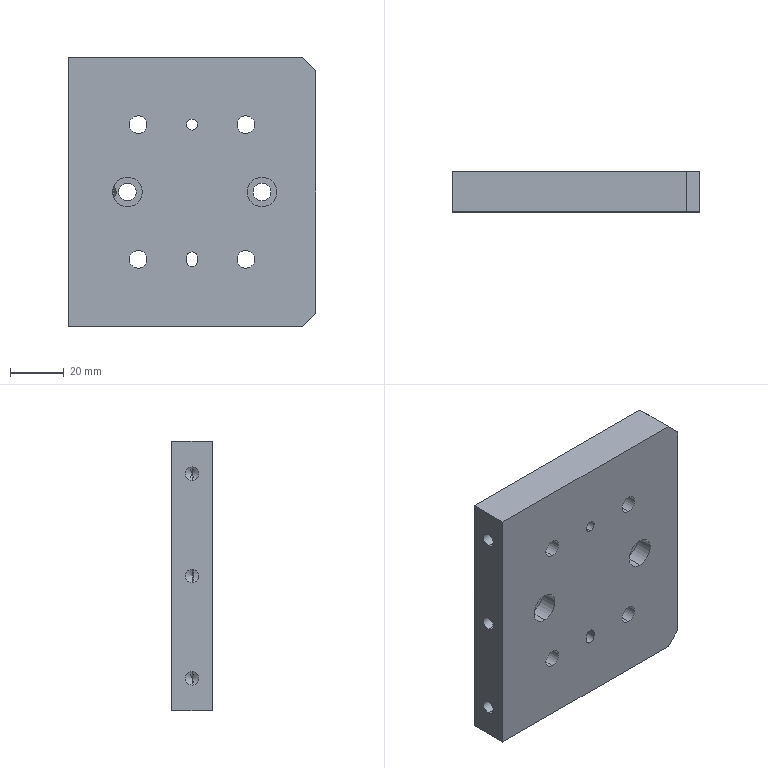Part | STEP file | PN_0019 | 1 solid | 57 faces | box 92 x 15 x 100 mm | volume 130571 mm3 | cylinder 35 | plane 16 | cone 6 | commonest cylinder face diameters 6.6 x12 11 x12 5 x6 4 x5